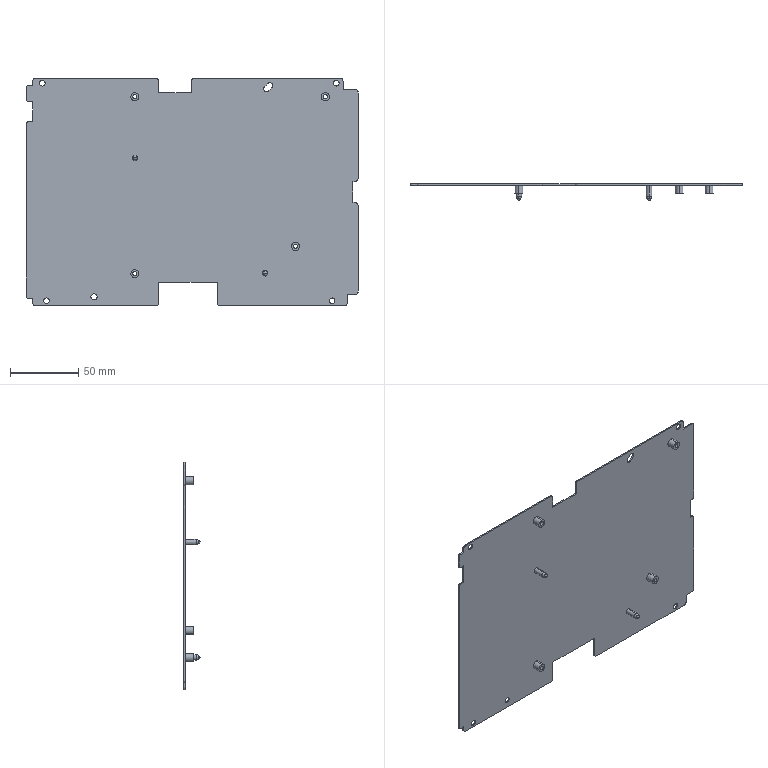Part | SolidWorks | features BaseBody 1 | 1 solid | 93 faces | box 244 x 12 x 167 mm | volume 40036 mm3 | cylinder 49 | plane 36 | cone 4 | spline 4 | commonest cylinder face diameters 4 x20 3 x8 4.2 x8 6 x8 4.5 x5